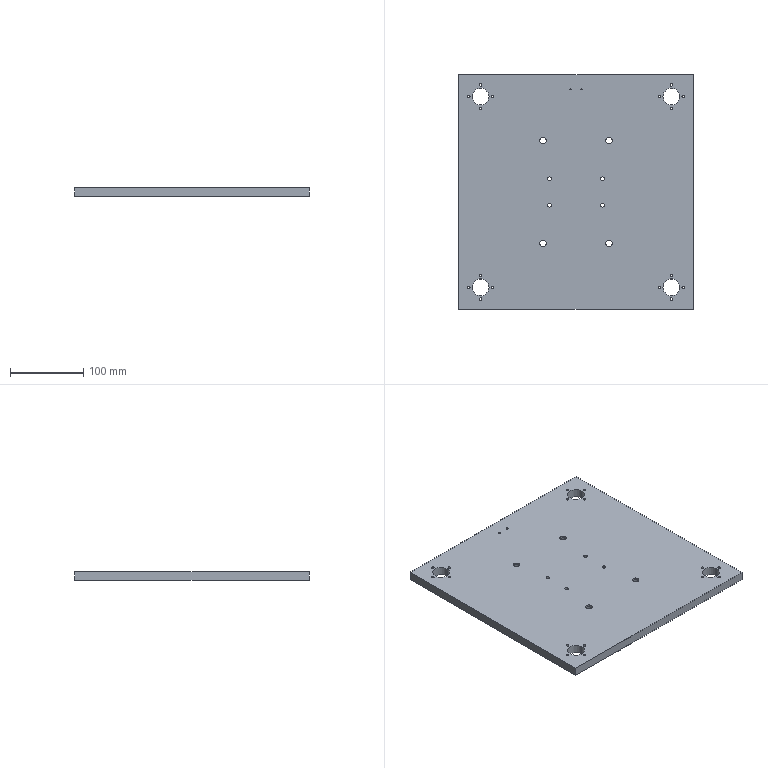Part | SolidWorks | features HoleWzd 4, MirrorPattern 2, Extrusion 1 | 1 solid | 82 faces | box 320 x 320 x 12 mm | volume 1198946 mm3 | cylinder 68 | plane 10 | cone 4 | commonest cylinder face diameters 3.3 x36 5 x8 9 x8 15 x8 23 x8